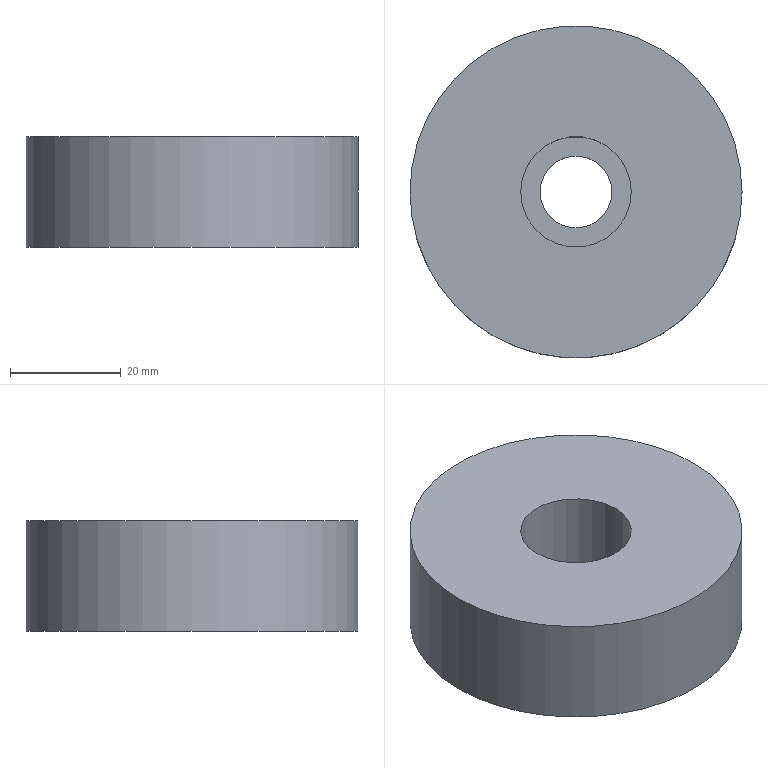Part | NX | features solid 2 | 1 solid | 6 faces | box 60 x 60 x 20 mm | volume 51354 mm3 | cylinder 3 | plane 3 | commonest cylinder face diameters 13 x1 20 x1 60 x1
STEP:
#1=CARTESIAN_POINT('',(-570.,-285.,25.));
#2=VERTEX_POINT('',#1);
#3=CARTESIAN_POINT('',(-600.,-285.,25.));
#4=DIRECTION('',(0.,0.,1.));
#5=DIRECTION('',(1.,0.,0.));
#6=AXIS2_PLACEMENT_3D('',#3,#4,#5);
#7=CIRCLE('',#6,30.);
#8=EDGE_CURVE('',#2,#2,#7,.T.);
#9=ORIENTED_EDGE('',*,*,#8,.F.);
#10=EDGE_LOOP('',(#9));
#11=FACE_BOUND('',#10,.T.);
#12=CARTESIAN_POINT('',(-570.,-285.,5.));
#13=VERTEX_POINT('',#12);
#14=CARTESIAN_POINT('',(-600.,-285.,5.));
#15=DIRECTION('',(0.,0.,1.));
#16=DIRECTION('',(1.,0.,0.));
#17=AXIS2_PLACEMENT_3D('',#14,#15,#16);
#18=CIRCLE('',#17,30.);
#19=EDGE_CURVE('',#13,#13,#18,.T.);
#20=ORIENTED_EDGE('',*,*,#19,.T.);
#21=EDGE_LOOP('',(#20));
#22=FACE_BOUND('',#21,.T.);
#23=CARTESIAN_POINT('',(-600.,-285.,25.));
#24=DIRECTION('',(0.,0.,-1.));
#25=DIRECTION('',(-1.,0.,0.));
#26=AXIS2_PLACEMENT_3D('',#23,#24,#25);
#27=CYLINDRICAL_SURFACE('',#26,30.);
#28=ADVANCED_FACE('',(#11,#22),#27,.T.);
#29=CARTESIAN_POINT('',(-610.,-285.,25.));
#30=VERTEX_POINT('',#29);
#31=CARTESIAN_POINT('',(-600.,-285.,25.));
#32=DIRECTION('',(0.,0.,-1.));
#33=DIRECTION('',(-1.,0.,0.));
#34=AXIS2_PLACEMENT_3D('',#31,#32,#33);
#35=CIRCLE('',#34,10.);
#36=EDGE_CURVE('',#30,#30,#35,.T.);
#37=ORIENTED_EDGE('',*,*,#36,.T.);
#38=EDGE_LOOP('',(#37));
#39=FACE_BOUND('',#38,.T.);
#40=ORIENTED_EDGE('',*,*,#8,.T.);
#41=EDGE_LOOP('',(#40));
#42=FACE_BOUND('',#41,.T.);
#43=CARTESIAN_POINT('',(-600.,-285.,25.));
#44=DIRECTION('',(0.,0.,1.));
#45=DIRECTION('',(1.,0.,0.));
#46=AXIS2_PLACEMENT_3D('',#43,#44,#45);
#47=PLANE('',#46);
#48=ADVANCED_FACE('',(#39,#42),#47,.T.);
#49=CARTESIAN_POINT('',(-593.5,-285.,5.));
#50=VERTEX_POINT('',#49);
#51=CARTESIAN_POINT('',(-600.,-285.,5.));
#52=DIRECTION('',(0.,0.,1.));
#53=DIRECTION('',(1.,0.,0.));
#54=AXIS2_PLACEMENT_3D('',#51,#52,#53);
#55=CIRCLE('',#54,6.5);
#56=EDGE_CURVE('',#50,#50,#55,.T.);
#57=ORIENTED_EDGE('',*,*,#56,.T.);
#58=EDGE_LOOP('',(#57));
#59=FACE_BOUND('',#58,.T.);
#60=ORIENTED_EDGE('',*,*,#19,.F.);
#61=EDGE_LOOP('',(#60));
#62=FACE_BOUND('',#61,.T.);
#63=CARTESIAN_POINT('',(-600.,-285.,5.));
#64=DIRECTION('',(0.,0.,1.));
#65=DIRECTION('',(1.,0.,0.));
#66=AXIS2_PLACEMENT_3D('',#63,#64,#65);
#67=PLANE('',#66);
#68=ADVANCED_FACE('',(#59,#62),#67,.F.);
#69=CARTESIAN_POINT('',(-606.5,-285.,11.));
#70=VERTEX_POINT('',#69);
#71=CARTESIAN_POINT('',(-600.,-285.,11.));
#72=DIRECTION('',(0.,0.,-1.));
#73=DIRECTION('',(-1.,0.,0.));
#74=AXIS2_PLACEMENT_3D('',#71,#72,#73);
#75=CIRCLE('',#74,6.5);
#76=EDGE_CURVE('',#70,#70,#75,.T.);
#77=ORIENTED_EDGE('',*,*,#76,.F.);
#78=EDGE_LOOP('',(#77));
#79=FACE_BOUND('',#78,.T.);
#80=ORIENTED_EDGE('',*,*,#56,.F.);
#81=EDGE_LOOP('',(#80));
#82=FACE_BOUND('',#81,.T.);
#83=CARTESIAN_POINT('',(-600.,-285.,-25.));
#84=DIRECTION('',(0.,0.,-1.));
#85=DIRECTION('',(-1.,0.,0.));
#86=AXIS2_PLACEMENT_3D('',#83,#84,#85);
#87=CYLINDRICAL_SURFACE('',#86,6.5);
#88=ADVANCED_FACE('',(#79,#82),#87,.F.);
#89=ORIENTED_EDGE('',*,*,#76,.T.);
#90=EDGE_LOOP('',(#89));
#91=FACE_BOUND('',#90,.T.);
#92=CARTESIAN_POINT('',(-610.,-285.,11.));
#93=VERTEX_POINT('',#92);
#94=CARTESIAN_POINT('',(-600.,-285.,11.));
#95=DIRECTION('',(0.,0.,-1.));
#96=DIRECTION('',(-1.,0.,0.));
#97=AXIS2_PLACEMENT_3D('',#94,#95,#96);
#98=CIRCLE('',#97,10.);
#99=EDGE_CURVE('',#93,#93,#98,.T.);
#100=ORIENTED_EDGE('',*,*,#99,.F.);
#101=EDGE_LOOP('',(#100));
#102=FACE_BOUND('',#101,.T.);
#103=CARTESIAN_POINT('',(-600.,-285.,11.));
#104=DIRECTION('',(0.,0.,-1.));
#105=DIRECTION('',(-1.,0.,0.));
#106=AXIS2_PLACEMENT_3D('',#103,#104,#105);
#107=PLANE('',#106);
#108=ADVANCED_FACE('',(#91,#102),#107,.F.);
#109=ORIENTED_EDGE('',*,*,#99,.T.);
#110=EDGE_LOOP('',(#109));
#111=FACE_BOUND('',#110,.T.);
#112=ORIENTED_EDGE('',*,*,#36,.F.);
#113=EDGE_LOOP('',(#112));
#114=FACE_BOUND('',#113,.T.);
#115=CARTESIAN_POINT('',(-600.,-285.,25.));
#116=DIRECTION('',(0.,0.,-1.));
#117=DIRECTION('',(-1.,0.,0.));
#118=AXIS2_PLACEMENT_3D('',#115,#116,#117);
#119=CYLINDRICAL_SURFACE('',#118,10.);
#120=ADVANCED_FACE('',(#111,#114),#119,.F.);
#121=CLOSED_SHELL('',(#28,#48,#68,#88,#108,#120));
#122=MANIFOLD_SOLID_BREP('',#121);
#123=(LENGTH_UNIT()NAMED_UNIT(*)SI_UNIT(.MILLI.,.METRE.));
#124=UNCERTAINTY_MEASURE_WITH_UNIT(LENGTH_MEASURE(0.00001),#123,'','');
#125=(NAMED_UNIT(*)PLANE_ANGLE_UNIT()SI_UNIT($,.RADIAN.));
#126=(NAMED_UNIT(*)SI_UNIT($,.STERADIAN.)SOLID_ANGLE_UNIT());
#127=(GEOMETRIC_REPRESENTATION_CONTEXT(3)GLOBAL_UNCERTAINTY_ASSIGNED_CONTEXT((#124))GLOBAL_UNIT_ASSIGNED_CONTEXT((#123,#125,#126))REPRESENTATION_CONTEXT('',''));
#128=ADVANCED_BREP_SHAPE_REPRESENTATION('',(#122),#127);